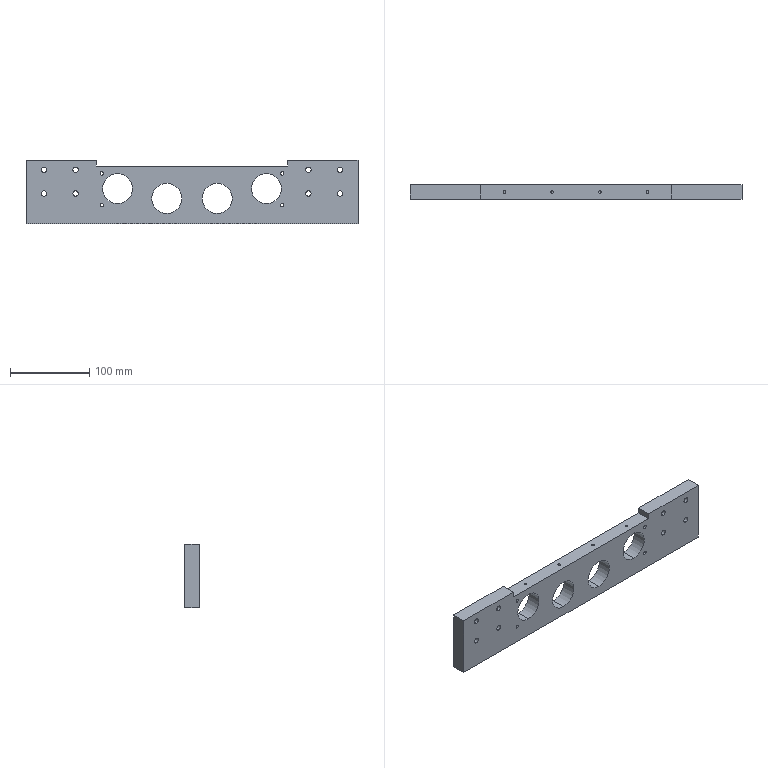Part | 1 solid | 98 faces | box 419 x 18 x 80 mm | volume 480420 mm3 | cylinder 62 | cone 26 | plane 10 | commonest cylinder face diameters 4.2 x24 6.8 x16 3.3 x8 38 x8 5 x6